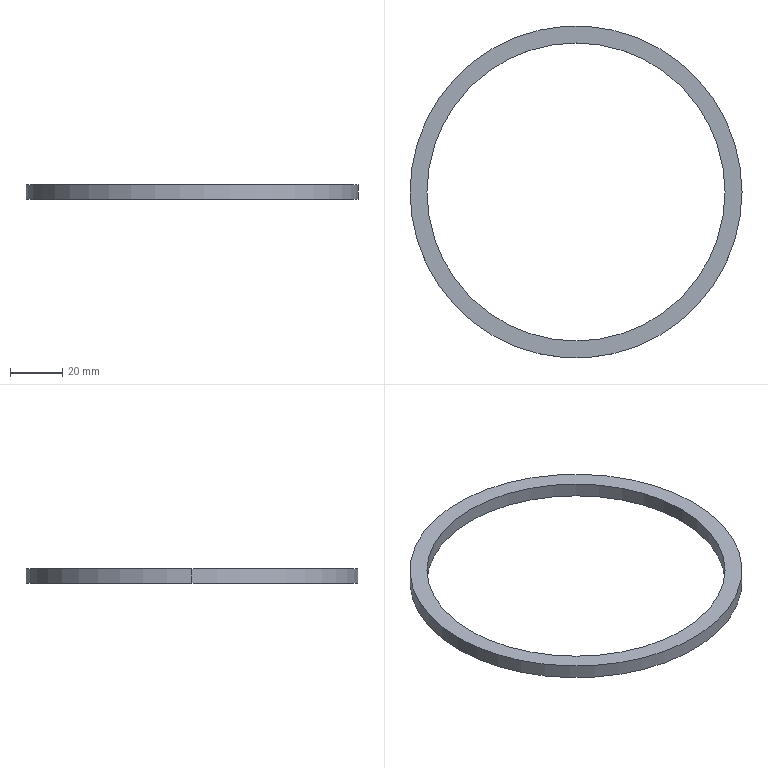Part | SolidWorks | features Extrusion 1 | 1 solid | 6 faces | box 127 x 127 x 5.5 mm | volume 13534 mm3 | cylinder 4 | plane 2 | commonest cylinder face diameters 114 x2 127 x2
STEP:
#1=CARTESIAN_POINT('',(-57.,0.,5.5));
#2=VERTEX_POINT('',#1);
#3=CARTESIAN_POINT('',(57.,0.,5.5));
#4=VERTEX_POINT('',#3);
#5=CARTESIAN_POINT('',(0.,0.,5.5));
#6=DIRECTION('',(0.,0.,1.));
#7=DIRECTION('',(1.,0.,0.));
#8=AXIS2_PLACEMENT_3D('',#5,#6,#7);
#9=CIRCLE('',#8,57.);
#10=EDGE_CURVE('',#2,#4,#9,.T.);
#11=ORIENTED_EDGE('',*,*,#10,.T.);
#12=CARTESIAN_POINT('',(57.,0.,0.));
#13=VERTEX_POINT('',#12);
#14=CARTESIAN_POINT('',(57.,0.,5.5));
#15=DIRECTION('',(0.,0.,-1.));
#16=VECTOR('',#15,1000.);
#17=LINE('',#14,#16);
#18=EDGE_CURVE('',#4,#13,#17,.T.);
#19=ORIENTED_EDGE('',*,*,#18,.T.);
#20=CARTESIAN_POINT('',(-57.,0.,0.));
#21=VERTEX_POINT('',#20);
#22=CARTESIAN_POINT('',(0.,0.,0.));
#23=DIRECTION('',(0.,0.,1.));
#24=DIRECTION('',(1.,0.,0.));
#25=AXIS2_PLACEMENT_3D('',#22,#23,#24);
#26=CIRCLE('',#25,57.);
#27=EDGE_CURVE('',#21,#13,#26,.T.);
#28=ORIENTED_EDGE('',*,*,#27,.F.);
#29=CARTESIAN_POINT('',(-57.,0.,5.5));
#30=DIRECTION('',(0.,0.,-1.));
#31=VECTOR('',#30,1000.);
#32=LINE('',#29,#31);
#33=EDGE_CURVE('',#2,#21,#32,.T.);
#34=ORIENTED_EDGE('',*,*,#33,.F.);
#35=EDGE_LOOP('',(#11,#19,#28,#34));
#36=FACE_OUTER_BOUND('',#35,.T.);
#37=CARTESIAN_POINT('',(0.,0.,5.5));
#38=DIRECTION('',(0.,0.,-1.));
#39=DIRECTION('',(-1.,0.,0.));
#40=AXIS2_PLACEMENT_3D('',#37,#38,#39);
#41=CYLINDRICAL_SURFACE('',#40,57.);
#42=ADVANCED_FACE('',(#36),#41,.F.);
#43=CARTESIAN_POINT('',(63.5,0.,5.5));
#44=VERTEX_POINT('',#43);
#45=CARTESIAN_POINT('',(-63.5,0.,5.5));
#46=VERTEX_POINT('',#45);
#47=CARTESIAN_POINT('',(0.,0.,5.5));
#48=DIRECTION('',(0.,0.,1.));
#49=DIRECTION('',(1.,0.,0.));
#50=AXIS2_PLACEMENT_3D('',#47,#48,#49);
#51=CIRCLE('',#50,63.5);
#52=EDGE_CURVE('',#44,#46,#51,.T.);
#53=ORIENTED_EDGE('',*,*,#52,.F.);
#54=CARTESIAN_POINT('',(63.5,0.,0.));
#55=VERTEX_POINT('',#54);
#56=CARTESIAN_POINT('',(63.5,0.,5.5));
#57=DIRECTION('',(0.,0.,-1.));
#58=VECTOR('',#57,1000.);
#59=LINE('',#56,#58);
#60=EDGE_CURVE('',#44,#55,#59,.T.);
#61=ORIENTED_EDGE('',*,*,#60,.T.);
#62=CARTESIAN_POINT('',(-63.5,0.,0.));
#63=VERTEX_POINT('',#62);
#64=CARTESIAN_POINT('',(0.,0.,0.));
#65=DIRECTION('',(0.,0.,1.));
#66=DIRECTION('',(1.,0.,0.));
#67=AXIS2_PLACEMENT_3D('',#64,#65,#66);
#68=CIRCLE('',#67,63.5);
#69=EDGE_CURVE('',#55,#63,#68,.T.);
#70=ORIENTED_EDGE('',*,*,#69,.T.);
#71=CARTESIAN_POINT('',(-63.5,0.,5.5));
#72=DIRECTION('',(0.,0.,-1.));
#73=VECTOR('',#72,1000.);
#74=LINE('',#71,#73);
#75=EDGE_CURVE('',#46,#63,#74,.T.);
#76=ORIENTED_EDGE('',*,*,#75,.F.);
#77=EDGE_LOOP('',(#53,#61,#70,#76));
#78=FACE_OUTER_BOUND('',#77,.T.);
#79=CARTESIAN_POINT('',(0.,0.,5.5));
#80=DIRECTION('',(0.,0.,-1.));
#81=DIRECTION('',(-1.,0.,0.));
#82=AXIS2_PLACEMENT_3D('',#79,#80,#81);
#83=CYLINDRICAL_SURFACE('',#82,63.5);
#84=ADVANCED_FACE('',(#78),#83,.T.);
#85=CARTESIAN_POINT('',(0.,0.,5.5));
#86=DIRECTION('',(0.,0.,1.));
#87=DIRECTION('',(1.,0.,0.));
#88=AXIS2_PLACEMENT_3D('',#85,#86,#87);
#89=CIRCLE('',#88,63.5);
#90=EDGE_CURVE('',#46,#44,#89,.T.);
#91=ORIENTED_EDGE('',*,*,#90,.T.);
#92=ORIENTED_EDGE('',*,*,#52,.T.);
#93=EDGE_LOOP('',(#91,#92));
#94=FACE_OUTER_BOUND('',#93,.T.);
#95=ORIENTED_EDGE('',*,*,#10,.F.);
#96=CARTESIAN_POINT('',(0.,0.,5.5));
#97=DIRECTION('',(0.,0.,1.));
#98=DIRECTION('',(1.,0.,0.));
#99=AXIS2_PLACEMENT_3D('',#96,#97,#98);
#100=CIRCLE('',#99,57.);
#101=EDGE_CURVE('',#4,#2,#100,.T.);
#102=ORIENTED_EDGE('',*,*,#101,.F.);
#103=EDGE_LOOP('',(#95,#102));
#104=FACE_BOUND('',#103,.T.);
#105=CARTESIAN_POINT('',(0.,0.,5.5));
#106=DIRECTION('',(0.,0.,1.));
#107=DIRECTION('',(1.,0.,0.));
#108=AXIS2_PLACEMENT_3D('',#105,#106,#107);
#109=PLANE('',#108);
#110=ADVANCED_FACE('',(#94,#104),#109,.T.);
#111=CARTESIAN_POINT('',(0.,0.,0.));
#112=DIRECTION('',(0.,0.,1.));
#113=DIRECTION('',(1.,0.,0.));
#114=AXIS2_PLACEMENT_3D('',#111,#112,#113);
#115=CIRCLE('',#114,63.5);
#116=EDGE_CURVE('',#63,#55,#115,.T.);
#117=ORIENTED_EDGE('',*,*,#116,.F.);
#118=ORIENTED_EDGE('',*,*,#69,.F.);
#119=EDGE_LOOP('',(#117,#118));
#120=FACE_OUTER_BOUND('',#119,.T.);
#121=ORIENTED_EDGE('',*,*,#27,.T.);
#122=CARTESIAN_POINT('',(0.,0.,0.));
#123=DIRECTION('',(0.,0.,1.));
#124=DIRECTION('',(1.,0.,0.));
#125=AXIS2_PLACEMENT_3D('',#122,#123,#124);
#126=CIRCLE('',#125,57.);
#127=EDGE_CURVE('',#13,#21,#126,.T.);
#128=ORIENTED_EDGE('',*,*,#127,.T.);
#129=EDGE_LOOP('',(#121,#128));
#130=FACE_BOUND('',#129,.T.);
#131=CARTESIAN_POINT('',(0.,0.,0.));
#132=DIRECTION('',(0.,0.,1.));
#133=DIRECTION('',(1.,0.,0.));
#134=AXIS2_PLACEMENT_3D('',#131,#132,#133);
#135=PLANE('',#134);
#136=ADVANCED_FACE('',(#120,#130),#135,.F.);
#137=ORIENTED_EDGE('',*,*,#60,.F.);
#138=ORIENTED_EDGE('',*,*,#90,.F.);
#139=ORIENTED_EDGE('',*,*,#75,.T.);
#140=ORIENTED_EDGE('',*,*,#116,.T.);
#141=EDGE_LOOP('',(#137,#138,#139,#140));
#142=FACE_OUTER_BOUND('',#141,.T.);
#143=CARTESIAN_POINT('',(0.,0.,5.5));
#144=DIRECTION('',(0.,0.,-1.));
#145=DIRECTION('',(-1.,0.,0.));
#146=AXIS2_PLACEMENT_3D('',#143,#144,#145);
#147=CYLINDRICAL_SURFACE('',#146,63.5);
#148=ADVANCED_FACE('',(#142),#147,.T.);
#149=ORIENTED_EDGE('',*,*,#18,.F.);
#150=ORIENTED_EDGE('',*,*,#101,.T.);
#151=ORIENTED_EDGE('',*,*,#33,.T.);
#152=ORIENTED_EDGE('',*,*,#127,.F.);
#153=EDGE_LOOP('',(#149,#150,#151,#152));
#154=FACE_OUTER_BOUND('',#153,.T.);
#155=CARTESIAN_POINT('',(0.,0.,5.5));
#156=DIRECTION('',(0.,0.,-1.));
#157=DIRECTION('',(-1.,0.,0.));
#158=AXIS2_PLACEMENT_3D('',#155,#156,#157);
#159=CYLINDRICAL_SURFACE('',#158,57.);
#160=ADVANCED_FACE('',(#154),#159,.F.);
#161=CLOSED_SHELL('',(#42,#84,#110,#136,#148,#160));
#162=MANIFOLD_SOLID_BREP('',#161);
#163=CARTESIAN_POINT('',(0.,0.,0.));
#164=DIRECTION('',(0.,0.,1.));
#165=DIRECTION('',(1.,0.,0.));
#166=AXIS2_PLACEMENT_3D('',#163,#164,#165);
#167=(LENGTH_UNIT()NAMED_UNIT(*)SI_UNIT(.MILLI.,.METRE.));
#168=UNCERTAINTY_MEASURE_WITH_UNIT(LENGTH_MEASURE(0.00001),#167,'','');
#169=(NAMED_UNIT(*)PLANE_ANGLE_UNIT()SI_UNIT($,.RADIAN.));
#170=(NAMED_UNIT(*)SI_UNIT($,.STERADIAN.)SOLID_ANGLE_UNIT());
#171=(GEOMETRIC_REPRESENTATION_CONTEXT(3)GLOBAL_UNCERTAINTY_ASSIGNED_CONTEXT((#168))GLOBAL_UNIT_ASSIGNED_CONTEXT((#167,#169,#170))REPRESENTATION_CONTEXT('',''));
#172=ADVANCED_BREP_SHAPE_REPRESENTATION('',(#162,#166),#171);